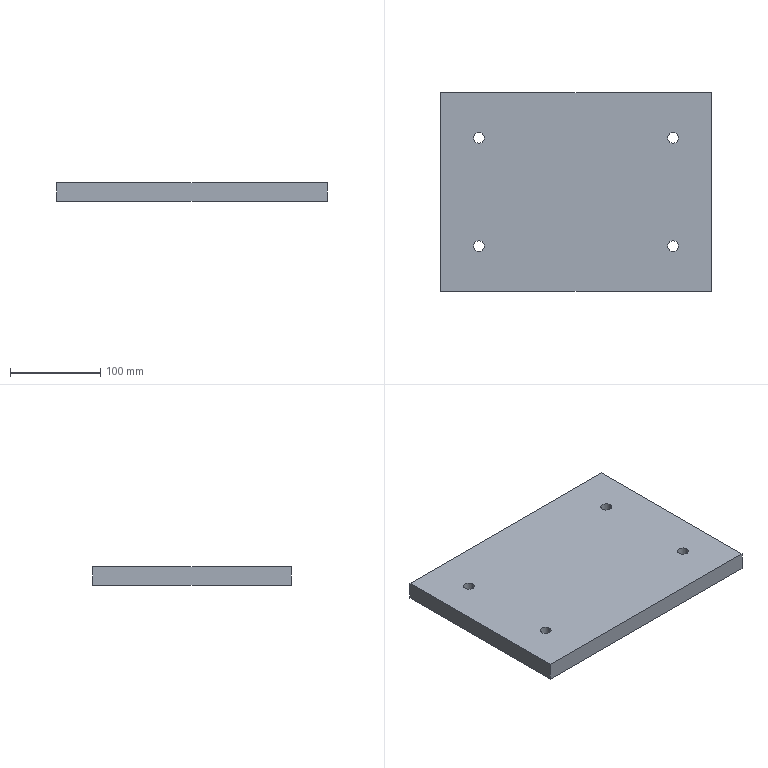Part | STEP file | 000 | 1 solid | 14 faces | box 300 x 220 x 20 mm | volume 1310952 mm3 | cylinder 8 | plane 6 | commonest cylinder face diameters 12 x8
STEP:
#1=CARTESIAN_POINT('',(0.,0.,0.));
#2=DIRECTION('',(0.,0.,1.));
#3=DIRECTION('',(1.,0.,0.));
#4=AXIS2_PLACEMENT_3D('',#1,#2,#3);
#5=CARTESIAN_POINT('',(-150.,110.,0.));
#6=VERTEX_POINT('',#5);
#7=CARTESIAN_POINT('',(-150.,-110.,0.));
#8=VERTEX_POINT('',#7);
#9=CARTESIAN_POINT('',(-150.,110.,0.));
#10=DIRECTION('',(0.,-1.,0.));
#11=VECTOR('',#10,1.);
#12=LINE('',#9,#11);
#13=CARTESIAN_POINT('',(0.,0.,0.));
#14=DIRECTION('',(0.,0.,1.));
#15=DIRECTION('',(1.,0.,0.));
#16=AXIS2_PLACEMENT_3D('',#13,#14,#15);
#17=PLANE('',#16);
#18=CARTESIAN_POINT('',(-150.,110.));
#19=DIRECTION('',(0.,-1.));
#20=VECTOR('',#19,1.);
#21=LINE('',#18,#20);
#22=(GEOMETRIC_REPRESENTATION_CONTEXT(2)PARAMETRIC_REPRESENTATION_CONTEXT()REPRESENTATION_CONTEXT('',''));
#23=DEFINITIONAL_REPRESENTATION('',(#21),#22);
#24=PCURVE('',#17,#23);
#25=CARTESIAN_POINT('',(-150.,0.,10.));
#26=DIRECTION('',(1.,0.,0.));
#27=DIRECTION('',(0.,-1.,0.));
#28=AXIS2_PLACEMENT_3D('',#25,#26,#27);
#29=PLANE('',#28);
#30=CARTESIAN_POINT('',(-110.,10.));
#31=DIRECTION('',(1.,0.));
#32=VECTOR('',#31,1.);
#33=LINE('',#30,#32);
#34=(GEOMETRIC_REPRESENTATION_CONTEXT(2)PARAMETRIC_REPRESENTATION_CONTEXT()REPRESENTATION_CONTEXT('',''));
#35=DEFINITIONAL_REPRESENTATION('',(#33),#34);
#36=PCURVE('',#29,#35);
#37=SURFACE_CURVE('',#12,(#24,#36),.PCURVE_S1.);
#38=EDGE_CURVE('',#6,#8,#37,.T.);
#39=ORIENTED_EDGE('',*,*,#38,.T.);
#40=CARTESIAN_POINT('',(150.,-110.,0.));
#41=VERTEX_POINT('',#40);
#42=CARTESIAN_POINT('',(-150.,-110.,0.));
#43=DIRECTION('',(1.,0.,0.));
#44=VECTOR('',#43,1.);
#45=LINE('',#42,#44);
#46=CARTESIAN_POINT('',(-150.,-110.));
#47=DIRECTION('',(1.,0.));
#48=VECTOR('',#47,1.);
#49=LINE('',#46,#48);
#50=(GEOMETRIC_REPRESENTATION_CONTEXT(2)PARAMETRIC_REPRESENTATION_CONTEXT()REPRESENTATION_CONTEXT('',''));
#51=DEFINITIONAL_REPRESENTATION('',(#49),#50);
#52=PCURVE('',#17,#51);
#53=CARTESIAN_POINT('',(0.,-110.,10.));
#54=DIRECTION('',(0.,1.,0.));
#55=DIRECTION('',(1.,0.,0.));
#56=AXIS2_PLACEMENT_3D('',#53,#54,#55);
#57=PLANE('',#56);
#58=CARTESIAN_POINT('',(-150.,10.));
#59=DIRECTION('',(1.,0.));
#60=VECTOR('',#59,1.);
#61=LINE('',#58,#60);
#62=(GEOMETRIC_REPRESENTATION_CONTEXT(2)PARAMETRIC_REPRESENTATION_CONTEXT()REPRESENTATION_CONTEXT('',''));
#63=DEFINITIONAL_REPRESENTATION('',(#61),#62);
#64=PCURVE('',#57,#63);
#65=SURFACE_CURVE('',#45,(#52,#64),.PCURVE_S1.);
#66=EDGE_CURVE('',#8,#41,#65,.T.);
#67=ORIENTED_EDGE('',*,*,#66,.T.);
#68=CARTESIAN_POINT('',(150.,110.,0.));
#69=VERTEX_POINT('',#68);
#70=CARTESIAN_POINT('',(150.,-110.,0.));
#71=DIRECTION('',(0.,1.,0.));
#72=VECTOR('',#71,1.);
#73=LINE('',#70,#72);
#74=CARTESIAN_POINT('',(150.,-110.));
#75=DIRECTION('',(0.,1.));
#76=VECTOR('',#75,1.);
#77=LINE('',#74,#76);
#78=(GEOMETRIC_REPRESENTATION_CONTEXT(2)PARAMETRIC_REPRESENTATION_CONTEXT()REPRESENTATION_CONTEXT('',''));
#79=DEFINITIONAL_REPRESENTATION('',(#77),#78);
#80=PCURVE('',#17,#79);
#81=CARTESIAN_POINT('',(150.,0.,10.));
#82=DIRECTION('',(-1.,0.,0.));
#83=DIRECTION('',(0.,1.,0.));
#84=AXIS2_PLACEMENT_3D('',#81,#82,#83);
#85=PLANE('',#84);
#86=CARTESIAN_POINT('',(-110.,10.));
#87=DIRECTION('',(1.,0.));
#88=VECTOR('',#87,1.);
#89=LINE('',#86,#88);
#90=(GEOMETRIC_REPRESENTATION_CONTEXT(2)PARAMETRIC_REPRESENTATION_CONTEXT()REPRESENTATION_CONTEXT('',''));
#91=DEFINITIONAL_REPRESENTATION('',(#89),#90);
#92=PCURVE('',#85,#91);
#93=SURFACE_CURVE('',#73,(#80,#92),.PCURVE_S1.);
#94=EDGE_CURVE('',#41,#69,#93,.T.);
#95=ORIENTED_EDGE('',*,*,#94,.T.);
#96=CARTESIAN_POINT('',(150.,110.,0.));
#97=DIRECTION('',(-1.,0.,0.));
#98=VECTOR('',#97,1.);
#99=LINE('',#96,#98);
#100=CARTESIAN_POINT('',(150.,110.));
#101=DIRECTION('',(-1.,0.));
#102=VECTOR('',#101,1.);
#103=LINE('',#100,#102);
#104=(GEOMETRIC_REPRESENTATION_CONTEXT(2)PARAMETRIC_REPRESENTATION_CONTEXT()REPRESENTATION_CONTEXT('',''));
#105=DEFINITIONAL_REPRESENTATION('',(#103),#104);
#106=PCURVE('',#17,#105);
#107=CARTESIAN_POINT('',(0.,110.,10.));
#108=DIRECTION('',(0.,-1.,0.));
#109=DIRECTION('',(-1.,0.,0.));
#110=AXIS2_PLACEMENT_3D('',#107,#108,#109);
#111=PLANE('',#110);
#112=CARTESIAN_POINT('',(-150.,10.));
#113=DIRECTION('',(1.,0.));
#114=VECTOR('',#113,1.);
#115=LINE('',#112,#114);
#116=(GEOMETRIC_REPRESENTATION_CONTEXT(2)PARAMETRIC_REPRESENTATION_CONTEXT()REPRESENTATION_CONTEXT('',''));
#117=DEFINITIONAL_REPRESENTATION('',(#115),#116);
#118=PCURVE('',#111,#117);
#119=SURFACE_CURVE('',#99,(#106,#118),.PCURVE_S1.);
#120=EDGE_CURVE('',#69,#6,#119,.T.);
#121=ORIENTED_EDGE('',*,*,#120,.T.);
#122=EDGE_LOOP('',(#39,#67,#95,#121));
#123=FACE_BOUND('',#122,.F.);
#124=CARTESIAN_POINT('',(-113.5,60.,0.));
#125=VERTEX_POINT('',#124);
#126=CARTESIAN_POINT('',(-101.5,60.,0.));
#127=VERTEX_POINT('',#126);
#128=CARTESIAN_POINT('',(-107.5,60.,0.));
#129=DIRECTION('',(0.,0.,-1.));
#130=DIRECTION('',(-1.,0.,0.));
#131=AXIS2_PLACEMENT_3D('',#128,#129,#130);
#132=CIRCLE('',#131,6.);
#133=CARTESIAN_POINT('',(-113.5,60.));
#134=CARTESIAN_POINT('',(-113.5,70.392));
#135=CARTESIAN_POINT('',(-104.5,65.196));
#136=CARTESIAN_POINT('',(-95.5,60.));
#137=CARTESIAN_POINT('',(-104.5,54.804));
#138=CARTESIAN_POINT('',(-113.5,49.608));
#139=CARTESIAN_POINT('',(-113.5,60.));
#140=(BOUNDED_CURVE()B_SPLINE_CURVE(2,(#133,#134,#135,#136,#137,#138,#139),.UNSPECIFIED.,.T.,.F.)B_SPLINE_CURVE_WITH_KNOTS((1,2,2,2,2,1),(-2.094,0.,2.094,4.189,6.283,8.378),.UNSPECIFIED.)CURVE()GEOMETRIC_REPRESENTATION_ITEM()RATIONAL_B_SPLINE_CURVE((1.,0.5,1.,0.5,1.,0.5,1.))REPRESENTATION_ITEM(''));
#141=(GEOMETRIC_REPRESENTATION_CONTEXT(2)PARAMETRIC_REPRESENTATION_CONTEXT()REPRESENTATION_CONTEXT('',''));
#142=DEFINITIONAL_REPRESENTATION('',(#140),#141);
#143=PCURVE('',#17,#142);
#144=CARTESIAN_POINT('',(-107.5,60.,20.));
#145=DIRECTION('',(0.,0.,-1.));
#146=DIRECTION('',(-1.,0.,0.));
#147=AXIS2_PLACEMENT_3D('',#144,#145,#146);
#148=CYLINDRICAL_SURFACE('',#147,6.);
#149=CARTESIAN_POINT('',(0.,20.));
#150=DIRECTION('',(1.,0.));
#151=VECTOR('',#150,1.);
#152=LINE('',#149,#151);
#153=(GEOMETRIC_REPRESENTATION_CONTEXT(2)PARAMETRIC_REPRESENTATION_CONTEXT()REPRESENTATION_CONTEXT('',''));
#154=DEFINITIONAL_REPRESENTATION('',(#152),#153);
#155=PCURVE('',#148,#154);
#156=SURFACE_CURVE('',#132,(#143,#155),.PCURVE_S1.);
#157=EDGE_CURVE('',#125,#127,#156,.T.);
#158=ORIENTED_EDGE('',*,*,#157,.T.);
#159=CARTESIAN_POINT('',(-107.5,60.,0.));
#160=DIRECTION('',(0.,0.,-1.));
#161=DIRECTION('',(1.,0.,0.));
#162=AXIS2_PLACEMENT_3D('',#159,#160,#161);
#163=CIRCLE('',#162,6.);
#164=CARTESIAN_POINT('',(-101.5,60.));
#165=CARTESIAN_POINT('',(-101.5,49.608));
#166=CARTESIAN_POINT('',(-110.5,54.804));
#167=CARTESIAN_POINT('',(-119.5,60.));
#168=CARTESIAN_POINT('',(-110.5,65.196));
#169=CARTESIAN_POINT('',(-101.5,70.392));
#170=CARTESIAN_POINT('',(-101.5,60.));
#171=(BOUNDED_CURVE()B_SPLINE_CURVE(2,(#164,#165,#166,#167,#168,#169,#170),.UNSPECIFIED.,.T.,.F.)B_SPLINE_CURVE_WITH_KNOTS((1,2,2,2,2,1),(-2.094,0.,2.094,4.189,6.283,8.378),.UNSPECIFIED.)CURVE()GEOMETRIC_REPRESENTATION_ITEM()RATIONAL_B_SPLINE_CURVE((1.,0.5,1.,0.5,1.,0.5,1.))REPRESENTATION_ITEM(''));
#172=(GEOMETRIC_REPRESENTATION_CONTEXT(2)PARAMETRIC_REPRESENTATION_CONTEXT()REPRESENTATION_CONTEXT('',''));
#173=DEFINITIONAL_REPRESENTATION('',(#171),#172);
#174=PCURVE('',#17,#173);
#175=CARTESIAN_POINT('',(-107.5,60.,20.));
#176=DIRECTION('',(0.,0.,-1.));
#177=DIRECTION('',(-1.,0.,0.));
#178=AXIS2_PLACEMENT_3D('',#175,#176,#177);
#179=CYLINDRICAL_SURFACE('',#178,6.);
#180=CARTESIAN_POINT('',(3.142,20.));
#181=DIRECTION('',(1.,0.));
#182=VECTOR('',#181,1.);
#183=LINE('',#180,#182);
#184=(GEOMETRIC_REPRESENTATION_CONTEXT(2)PARAMETRIC_REPRESENTATION_CONTEXT()REPRESENTATION_CONTEXT('',''));
#185=DEFINITIONAL_REPRESENTATION('',(#183),#184);
#186=PCURVE('',#179,#185);
#187=SURFACE_CURVE('',#163,(#174,#186),.PCURVE_S1.);
#188=EDGE_CURVE('',#127,#125,#187,.T.);
#189=ORIENTED_EDGE('',*,*,#188,.T.);
#190=EDGE_LOOP('',(#158,#189));
#191=FACE_BOUND('',#190,.F.);
#192=CARTESIAN_POINT('',(101.5,60.,0.));
#193=VERTEX_POINT('',#192);
#194=CARTESIAN_POINT('',(113.5,60.,0.));
#195=VERTEX_POINT('',#194);
#196=CARTESIAN_POINT('',(107.5,60.,0.));
#197=DIRECTION('',(0.,0.,-1.));
#198=DIRECTION('',(-1.,0.,0.));
#199=AXIS2_PLACEMENT_3D('',#196,#197,#198);
#200=CIRCLE('',#199,6.);
#201=CARTESIAN_POINT('',(101.5,60.));
#202=CARTESIAN_POINT('',(101.5,70.392));
#203=CARTESIAN_POINT('',(110.5,65.196));
#204=CARTESIAN_POINT('',(119.5,60.));
#205=CARTESIAN_POINT('',(110.5,54.804));
#206=CARTESIAN_POINT('',(101.5,49.608));
#207=CARTESIAN_POINT('',(101.5,60.));
#208=(BOUNDED_CURVE()B_SPLINE_CURVE(2,(#201,#202,#203,#204,#205,#206,#207),.UNSPECIFIED.,.T.,.F.)B_SPLINE_CURVE_WITH_KNOTS((1,2,2,2,2,1),(-2.094,0.,2.094,4.189,6.283,8.378),.UNSPECIFIED.)CURVE()GEOMETRIC_REPRESENTATION_ITEM()RATIONAL_B_SPLINE_CURVE((1.,0.5,1.,0.5,1.,0.5,1.))REPRESENTATION_ITEM(''));
#209=(GEOMETRIC_REPRESENTATION_CONTEXT(2)PARAMETRIC_REPRESENTATION_CONTEXT()REPRESENTATION_CONTEXT('',''));
#210=DEFINITIONAL_REPRESENTATION('',(#208),#209);
#211=PCURVE('',#17,#210);
#212=CARTESIAN_POINT('',(107.5,60.,20.));
#213=DIRECTION('',(0.,0.,-1.));
#214=DIRECTION('',(-1.,0.,0.));
#215=AXIS2_PLACEMENT_3D('',#212,#213,#214);
#216=CYLINDRICAL_SURFACE('',#215,6.);
#217=CARTESIAN_POINT('',(0.,20.));
#218=DIRECTION('',(1.,0.));
#219=VECTOR('',#218,1.);
#220=LINE('',#217,#219);
#221=(GEOMETRIC_REPRESENTATION_CONTEXT(2)PARAMETRIC_REPRESENTATION_CONTEXT()REPRESENTATION_CONTEXT('',''));
#222=DEFINITIONAL_REPRESENTATION('',(#220),#221);
#223=PCURVE('',#216,#222);
#224=SURFACE_CURVE('',#200,(#211,#223),.PCURVE_S1.);
#225=EDGE_CURVE('',#193,#195,#224,.T.);
#226=ORIENTED_EDGE('',*,*,#225,.T.);
#227=CARTESIAN_POINT('',(107.5,60.,0.));
#228=DIRECTION('',(0.,0.,-1.));
#229=DIRECTION('',(1.,0.,0.));
#230=AXIS2_PLACEMENT_3D('',#227,#228,#229);
#231=CIRCLE('',#230,6.);
#232=CARTESIAN_POINT('',(113.5,60.));
#233=CARTESIAN_POINT('',(113.5,49.608));
#234=CARTESIAN_POINT('',(104.5,54.804));
#235=CARTESIAN_POINT('',(95.5,60.));
#236=CARTESIAN_POINT('',(104.5,65.196));
#237=CARTESIAN_POINT('',(113.5,70.392));
#238=CARTESIAN_POINT('',(113.5,60.));
#239=(BOUNDED_CURVE()B_SPLINE_CURVE(2,(#232,#233,#234,#235,#236,#237,#238),.UNSPECIFIED.,.T.,.F.)B_SPLINE_CURVE_WITH_KNOTS((1,2,2,2,2,1),(-2.094,0.,2.094,4.189,6.283,8.378),.UNSPECIFIED.)CURVE()GEOMETRIC_REPRESENTATION_ITEM()RATIONAL_B_SPLINE_CURVE((1.,0.5,1.,0.5,1.,0.5,1.))REPRESENTATION_ITEM(''));
#240=(GEOMETRIC_REPRESENTATION_CONTEXT(2)PARAMETRIC_REPRESENTATION_CONTEXT()REPRESENTATION_CONTEXT('',''));
#241=DEFINITIONAL_REPRESENTATION('',(#239),#240);
#242=PCURVE('',#17,#241);
#243=CARTESIAN_POINT('',(107.5,60.,20.));
#244=DIRECTION('',(0.,0.,-1.));
#245=DIRECTION('',(-1.,0.,0.));
#246=AXIS2_PLACEMENT_3D('',#243,#244,#245);
#247=CYLINDRICAL_SURFACE('',#246,6.);
#248=CARTESIAN_POINT('',(3.142,20.));
#249=DIRECTION('',(1.,0.));
#250=VECTOR('',#249,1.);
#251=LINE('',#248,#250);
#252=(GEOMETRIC_REPRESENTATION_CONTEXT(2)PARAMETRIC_REPRESENTATION_CONTEXT()REPRESENTATION_CONTEXT('',''));
#253=DEFINITIONAL_REPRESENTATION('',(#251),#252);
#254=PCURVE('',#247,#253);
#255=SURFACE_CURVE('',#231,(#242,#254),.PCURVE_S1.);
#256=EDGE_CURVE('',#195,#193,#255,.T.);
#257=ORIENTED_EDGE('',*,*,#256,.T.);
#258=EDGE_LOOP('',(#226,#257));
#259=FACE_BOUND('',#258,.F.);
#260=CARTESIAN_POINT('',(-113.5,-60.,0.));
#261=VERTEX_POINT('',#260);
#262=CARTESIAN_POINT('',(-101.5,-60.,0.));
#263=VERTEX_POINT('',#262);
#264=CARTESIAN_POINT('',(-107.5,-60.,0.));
#265=DIRECTION('',(0.,0.,-1.));
#266=DIRECTION('',(-1.,0.,0.));
#267=AXIS2_PLACEMENT_3D('',#264,#265,#266);
#268=CIRCLE('',#267,6.);
#269=CARTESIAN_POINT('',(-113.5,-60.));
#270=CARTESIAN_POINT('',(-113.5,-49.608));
#271=CARTESIAN_POINT('',(-104.5,-54.804));
#272=CARTESIAN_POINT('',(-95.5,-60.));
#273=CARTESIAN_POINT('',(-104.5,-65.196));
#274=CARTESIAN_POINT('',(-113.5,-70.392));
#275=CARTESIAN_POINT('',(-113.5,-60.));
#276=(BOUNDED_CURVE()B_SPLINE_CURVE(2,(#269,#270,#271,#272,#273,#274,#275),.UNSPECIFIED.,.T.,.F.)B_SPLINE_CURVE_WITH_KNOTS((1,2,2,2,2,1),(-2.094,0.,2.094,4.189,6.283,8.378),.UNSPECIFIED.)CURVE()GEOMETRIC_REPRESENTATION_ITEM()RATIONAL_B_SPLINE_CURVE((1.,0.5,1.,0.5,1.,0.5,1.))REPRESENTATION_ITEM(''));
#277=(GEOMETRIC_REPRESENTATION_CONTEXT(2)PARAMETRIC_REPRESENTATION_CONTEXT()REPRESENTATION_CONTEXT('',''));
#278=DEFINITIONAL_REPRESENTATION('',(#276),#277);
#279=PCURVE('',#17,#278);
#280=CARTESIAN_POINT('',(-107.5,-60.,20.));
#281=DIRECTION('',(0.,0.,-1.));
#282=DIRECTION('',(-1.,0.,0.));
#283=AXIS2_PLACEMENT_3D('',#280,#281,#282);
#284=CYLINDRICAL_SURFACE('',#283,6.);
#285=CARTESIAN_POINT('',(0.,20.));
#286=DIRECTION('',(1.,0.));
#287=VECTOR('',#286,1.);
#288=LINE('',#285,#287);
#289=(GEOMETRIC_REPRESENTATION_CONTEXT(2)PARAMETRIC_REPRESENTATION_CONTEXT()REPRESENTATION_CONTEXT('',''));
#290=DEFINITIONAL_REPRESENTATION('',(#288),#289);
#291=PCURVE('',#284,#290);
#292=SURFACE_CURVE('',#268,(#279,#291),.PCURVE_S1.);
#293=EDGE_CURVE('',#261,#263,#292,.T.);
#294=ORIENTED_EDGE('',*,*,#293,.T.);
#295=CARTESIAN_POINT('',(-107.5,-60.,0.));
#296=DIRECTION('',(0.,0.,-1.));
#297=DIRECTION('',(1.,0.,0.));
#298=AXIS2_PLACEMENT_3D('',#295,#296,#297);
#299=CIRCLE('',#298,6.);
#300=CARTESIAN_POINT('',(-101.5,-60.));
#301=CARTESIAN_POINT('',(-101.5,-70.392));
#302=CARTESIAN_POINT('',(-110.5,-65.196));
#303=CARTESIAN_POINT('',(-119.5,-60.));
#304=CARTESIAN_POINT('',(-110.5,-54.804));
#305=CARTESIAN_POINT('',(-101.5,-49.608));
#306=CARTESIAN_POINT('',(-101.5,-60.));
#307=(BOUNDED_CURVE()B_SPLINE_CURVE(2,(#300,#301,#302,#303,#304,#305,#306),.UNSPECIFIED.,.T.,.F.)B_SPLINE_CURVE_WITH_KNOTS((1,2,2,2,2,1),(-2.094,0.,2.094,4.189,6.283,8.378),.UNSPECIFIED.)CURVE()GEOMETRIC_REPRESENTATION_ITEM()RATIONAL_B_SPLINE_CURVE((1.,0.5,1.,0.5,1.,0.5,1.))REPRESENTATION_ITEM(''));
#308=(GEOMETRIC_REPRESENTATION_CONTEXT(2)PARAMETRIC_REPRESENTATION_CONTEXT()REPRESENTATION_CONTEXT('',''));
#309=DEFINITIONAL_REPRESENTATION('',(#307),#308);
#310=PCURVE('',#17,#309);
#311=CARTESIAN_POINT('',(-107.5,-60.,20.));
#312=DIRECTION('',(0.,0.,-1.));
#313=DIRECTION('',(-1.,0.,0.));
#314=AXIS2_PLACEMENT_3D('',#311,#312,#313);
#315=CYLINDRICAL_SURFACE('',#314,6.);
#316=CARTESIAN_POINT('',(3.142,20.));
#317=DIRECTION('',(1.,0.));
#318=VECTOR('',#317,1.);
#319=LINE('',#316,#318);
#320=(GEOMETRIC_REPRESENTATION_CONTEXT(2)PARAMETRIC_REPRESENTATION_CONTEXT()REPRESENTATION_CONTEXT('',''));
#321=DEFINITIONAL_REPRESENTATION('',(#319),#320);
#322=PCURVE('',#315,#321);
#323=SURFACE_CURVE('',#299,(#310,#322),.PCURVE_S1.);
#324=EDGE_CURVE('',#263,#261,#323,.T.);
#325=ORIENTED_EDGE('',*,*,#324,.T.);
#326=EDGE_LOOP('',(#294,#325));
#327=FACE_BOUND('',#326,.F.);
#328=CARTESIAN_POINT('',(101.5,-60.,0.));
#329=VERTEX_POINT('',#328);
#330=CARTESIAN_POINT('',(113.5,-60.,0.));
#331=VERTEX_POINT('',#330);
#332=CARTESIAN_POINT('',(107.5,-60.,0.));
#333=DIRECTION('',(0.,0.,-1.));
#334=DIRECTION('',(-1.,0.,0.));
#335=AXIS2_PLACEMENT_3D('',#332,#333,#334);
#336=CIRCLE('',#335,6.);
#337=CARTESIAN_POINT('',(101.5,-60.));
#338=CARTESIAN_POINT('',(101.5,-49.608));
#339=CARTESIAN_POINT('',(110.5,-54.804));
#340=CARTESIAN_POINT('',(119.5,-60.));
#341=CARTESIAN_POINT('',(110.5,-65.196));
#342=CARTESIAN_POINT('',(101.5,-70.392));
#343=CARTESIAN_POINT('',(101.5,-60.));
#344=(BOUNDED_CURVE()B_SPLINE_CURVE(2,(#337,#338,#339,#340,#341,#342,#343),.UNSPECIFIED.,.T.,.F.)B_SPLINE_CURVE_WITH_KNOTS((1,2,2,2,2,1),(-2.094,0.,2.094,4.189,6.283,8.378),.UNSPECIFIED.)CURVE()GEOMETRIC_REPRESENTATION_ITEM()RATIONAL_B_SPLINE_CURVE((1.,0.5,1.,0.5,1.,0.5,1.))REPRESENTATION_ITEM(''));
#345=(GEOMETRIC_REPRESENTATION_CONTEXT(2)PARAMETRIC_REPRESENTATION_CONTEXT()REPRESENTATION_CONTEXT('',''));
#346=DEFINITIONAL_REPRESENTATION('',(#344),#345);
#347=PCURVE('',#17,#346);
#348=CARTESIAN_POINT('',(107.5,-60.,20.));
#349=DIRECTION('',(0.,0.,-1.));
#350=DIRECTION('',(-1.,0.,0.));
#351=AXIS2_PLACEMENT_3D('',#348,#349,#350);
#352=CYLINDRICAL_SURFACE('',#351,6.);
#353=CARTESIAN_POINT('',(0.,20.));
#354=DIRECTION('',(1.,0.));
#355=VECTOR('',#354,1.);
#356=LINE('',#353,#355);
#357=(GEOMETRIC_REPRESENTATION_CONTEXT(2)PARAMETRIC_REPRESENTATION_CONTEXT()REPRESENTATION_CONTEXT('',''));
#358=DEFINITIONAL_REPRESENTATION('',(#356),#357);
#359=PCURVE('',#352,#358);
#360=SURFACE_CURVE('',#336,(#347,#359),.PCURVE_S1.);
#361=EDGE_CURVE('',#329,#331,#360,.T.);
#362=ORIENTED_EDGE('',*,*,#361,.T.);
#363=CARTESIAN_POINT('',(107.5,-60.,0.));
#364=DIRECTION('',(0.,0.,-1.));
#365=DIRECTION('',(1.,0.,0.));
#366=AXIS2_PLACEMENT_3D('',#363,#364,#365);
#367=CIRCLE('',#366,6.);
#368=CARTESIAN_POINT('',(113.5,-60.));
#369=CARTESIAN_POINT('',(113.5,-70.392));
#370=CARTESIAN_POINT('',(104.5,-65.196));
#371=CARTESIAN_POINT('',(95.5,-60.));
#372=CARTESIAN_POINT('',(104.5,-54.804));
#373=CARTESIAN_POINT('',(113.5,-49.608));
#374=CARTESIAN_POINT('',(113.5,-60.));
#375=(BOUNDED_CURVE()B_SPLINE_CURVE(2,(#368,#369,#370,#371,#372,#373,#374),.UNSPECIFIED.,.T.,.F.)B_SPLINE_CURVE_WITH_KNOTS((1,2,2,2,2,1),(-2.094,0.,2.094,4.189,6.283,8.378),.UNSPECIFIED.)CURVE()GEOMETRIC_REPRESENTATION_ITEM()RATIONAL_B_SPLINE_CURVE((1.,0.5,1.,0.5,1.,0.5,1.))REPRESENTATION_ITEM(''));
#376=(GEOMETRIC_REPRESENTATION_CONTEXT(2)PARAMETRIC_REPRESENTATION_CONTEXT()REPRESENTATION_CONTEXT('',''));
#377=DEFINITIONAL_REPRESENTATION('',(#375),#376);
#378=PCURVE('',#17,#377);
#379=CARTESIAN_POINT('',(107.5,-60.,20.));
#380=DIRECTION('',(0.,0.,-1.));
#381=DIRECTION('',(-1.,0.,0.));
#382=AXIS2_PLACEMENT_3D('',#379,#380,#381);
#383=CYLINDRICAL_SURFACE('',#382,6.);
#384=CARTESIAN_POINT('',(3.142,20.));
#385=DIRECTION('',(1.,0.));
#386=VECTOR('',#385,1.);
#387=LINE('',#384,#386);
#388=(GEOMETRIC_REPRESENTATION_CONTEXT(2)PARAMETRIC_REPRESENTATION_CONTEXT()REPRESENTATION_CONTEXT('',''));
#389=DEFINITIONAL_REPRESENTATION('',(#387),#388);
#390=PCURVE('',#383,#389);
#391=SURFACE_CURVE('',#367,(#378,#390),.PCURVE_S1.);
#392=EDGE_CURVE('',#331,#329,#391,.T.);
#393=ORIENTED_EDGE('',*,*,#392,.T.);
#394=EDGE_LOOP('',(#362,#393));
#395=FACE_BOUND('',#394,.F.);
#396=ADVANCED_FACE('',(#123,#191,#259,#327,#395),#17,.F.);
#397=ORIENTED_EDGE('',*,*,#38,.F.);
#398=CARTESIAN_POINT('',(-150.,110.,20.));
#399=VERTEX_POINT('',#398);
#400=CARTESIAN_POINT('',(-150.,110.,0.));
#401=DIRECTION('',(0.,0.,1.));
#402=VECTOR('',#401,1.);
#403=LINE('',#400,#402);
#404=CARTESIAN_POINT('',(-110.,10.));
#405=DIRECTION('',(0.,-1.));
#406=VECTOR('',#405,1.);
#407=LINE('',#404,#406);
#408=(GEOMETRIC_REPRESENTATION_CONTEXT(2)PARAMETRIC_REPRESENTATION_CONTEXT()REPRESENTATION_CONTEXT('',''));
#409=DEFINITIONAL_REPRESENTATION('',(#407),#408);
#410=PCURVE('',#29,#409);
#411=CARTESIAN_POINT('',(150.,10.));
#412=DIRECTION('',(0.,-1.));
#413=VECTOR('',#412,1.);
#414=LINE('',#411,#413);
#415=(GEOMETRIC_REPRESENTATION_CONTEXT(2)PARAMETRIC_REPRESENTATION_CONTEXT()REPRESENTATION_CONTEXT('',''));
#416=DEFINITIONAL_REPRESENTATION('',(#414),#415);
#417=PCURVE('',#111,#416);
#418=SURFACE_CURVE('',#403,(#410,#417),.PCURVE_S1.);
#419=EDGE_CURVE('',#6,#399,#418,.T.);
#420=ORIENTED_EDGE('',*,*,#419,.T.);
#421=CARTESIAN_POINT('',(-150.,-110.,20.));
#422=VERTEX_POINT('',#421);
#423=CARTESIAN_POINT('',(-150.,110.,20.));
#424=DIRECTION('',(0.,-1.,0.));
#425=VECTOR('',#424,1.);
#426=LINE('',#423,#425);
#427=CARTESIAN_POINT('',(-110.,-10.));
#428=DIRECTION('',(1.,0.));
#429=VECTOR('',#428,1.);
#430=LINE('',#427,#429);
#431=(GEOMETRIC_REPRESENTATION_CONTEXT(2)PARAMETRIC_REPRESENTATION_CONTEXT()REPRESENTATION_CONTEXT('',''));
#432=DEFINITIONAL_REPRESENTATION('',(#430),#431);
#433=PCURVE('',#29,#432);
#434=CARTESIAN_POINT('',(0.,0.,20.));
#435=DIRECTION('',(0.,0.,1.));
#436=DIRECTION('',(1.,0.,0.));
#437=AXIS2_PLACEMENT_3D('',#434,#435,#436);
#438=PLANE('',#437);
#439=CARTESIAN_POINT('',(-150.,110.));
#440=DIRECTION('',(0.,-1.));
#441=VECTOR('',#440,1.);
#442=LINE('',#439,#441);
#443=(GEOMETRIC_REPRESENTATION_CONTEXT(2)PARAMETRIC_REPRESENTATION_CONTEXT()REPRESENTATION_CONTEXT('',''));
#444=DEFINITIONAL_REPRESENTATION('',(#442),#443);
#445=PCURVE('',#438,#444);
#446=SURFACE_CURVE('',#426,(#433,#445),.PCURVE_S1.);
#447=EDGE_CURVE('',#399,#422,#446,.T.);
#448=ORIENTED_EDGE('',*,*,#447,.T.);
#449=CARTESIAN_POINT('',(-150.,-110.,0.));
#450=DIRECTION('',(0.,0.,1.));
#451=VECTOR('',#450,1.);
#452=LINE('',#449,#451);
#453=CARTESIAN_POINT('',(110.,10.));
#454=DIRECTION('',(0.,-1.));
#455=VECTOR('',#454,1.);
#456=LINE('',#453,#455);
#457=(GEOMETRIC_REPRESENTATION_CONTEXT(2)PARAMETRIC_REPRESENTATION_CONTEXT()REPRESENTATION_CONTEXT('',''));
#458=DEFINITIONAL_REPRESENTATION('',(#456),#457);
#459=PCURVE('',#29,#458);
#460=CARTESIAN_POINT('',(-150.,10.));
#461=DIRECTION('',(0.,-1.));
#462=VECTOR('',#461,1.);
#463=LINE('',#460,#462);
#464=(GEOMETRIC_REPRESENTATION_CONTEXT(2)PARAMETRIC_REPRESENTATION_CONTEXT()REPRESENTATION_CONTEXT('',''));
#465=DEFINITIONAL_REPRESENTATION('',(#463),#464);
#466=PCURVE('',#57,#465);
#467=SURFACE_CURVE('',#452,(#459,#466),.PCURVE_S1.);
#468=EDGE_CURVE('',#8,#422,#467,.T.);
#469=ORIENTED_EDGE('',*,*,#468,.F.);
#470=EDGE_LOOP('',(#397,#420,#448,#469));
#471=FACE_BOUND('',#470,.F.);
#472=ADVANCED_FACE('',(#471),#29,.F.);
#473=ORIENTED_EDGE('',*,*,#120,.F.);
#474=CARTESIAN_POINT('',(150.,110.,20.));
#475=VERTEX_POINT('',#474);
#476=CARTESIAN_POINT('',(150.,110.,0.));
#477=DIRECTION('',(0.,0.,1.));
#478=VECTOR('',#477,1.);
#479=LINE('',#476,#478);
#480=CARTESIAN_POINT('',(-150.,10.));
#481=DIRECTION('',(0.,-1.));
#482=VECTOR('',#481,1.);
#483=LINE('',#480,#482);
#484=(GEOMETRIC_REPRESENTATION_CONTEXT(2)PARAMETRIC_REPRESENTATION_CONTEXT()REPRESENTATION_CONTEXT('',''));
#485=DEFINITIONAL_REPRESENTATION('',(#483),#484);
#486=PCURVE('',#111,#485);
#487=CARTESIAN_POINT('',(110.,10.));
#488=DIRECTION('',(0.,-1.));
#489=VECTOR('',#488,1.);
#490=LINE('',#487,#489);
#491=(GEOMETRIC_REPRESENTATION_CONTEXT(2)PARAMETRIC_REPRESENTATION_CONTEXT()REPRESENTATION_CONTEXT('',''));
#492=DEFINITIONAL_REPRESENTATION('',(#490),#491);
#493=PCURVE('',#85,#492);
#494=SURFACE_CURVE('',#479,(#486,#493),.PCURVE_S1.);
#495=EDGE_CURVE('',#69,#475,#494,.T.);
#496=ORIENTED_EDGE('',*,*,#495,.T.);
#497=CARTESIAN_POINT('',(150.,110.,20.));
#498=DIRECTION('',(-1.,0.,0.));
#499=VECTOR('',#498,1.);
#500=LINE('',#497,#499);
#501=CARTESIAN_POINT('',(-150.,-10.));
#502=DIRECTION('',(1.,0.));
#503=VECTOR('',#502,1.);
#504=LINE('',#501,#503);
#505=(GEOMETRIC_REPRESENTATION_CONTEXT(2)PARAMETRIC_REPRESENTATION_CONTEXT()REPRESENTATION_CONTEXT('',''));
#506=DEFINITIONAL_REPRESENTATION('',(#504),#505);
#507=PCURVE('',#111,#506);
#508=CARTESIAN_POINT('',(150.,110.));
#509=DIRECTION('',(-1.,0.));
#510=VECTOR('',#509,1.);
#511=LINE('',#508,#510);
#512=(GEOMETRIC_REPRESENTATION_CONTEXT(2)PARAMETRIC_REPRESENTATION_CONTEXT()REPRESENTATION_CONTEXT('',''));
#513=DEFINITIONAL_REPRESENTATION('',(#511),#512);
#514=PCURVE('',#438,#513);
#515=SURFACE_CURVE('',#500,(#507,#514),.PCURVE_S1.);
#516=EDGE_CURVE('',#475,#399,#515,.T.);
#517=ORIENTED_EDGE('',*,*,#516,.T.);
#518=ORIENTED_EDGE('',*,*,#419,.F.);
#519=EDGE_LOOP('',(#473,#496,#517,#518));
#520=FACE_BOUND('',#519,.F.);
#521=ADVANCED_FACE('',(#520),#111,.F.);
#522=ORIENTED_EDGE('',*,*,#94,.F.);
#523=CARTESIAN_POINT('',(150.,-110.,20.));
#524=VERTEX_POINT('',#523);
#525=CARTESIAN_POINT('',(150.,-110.,0.));
#526=DIRECTION('',(0.,0.,1.));
#527=VECTOR('',#526,1.);
#528=LINE('',#525,#527);
#529=CARTESIAN_POINT('',(-110.,10.));
#530=DIRECTION('',(0.,-1.));
#531=VECTOR('',#530,1.);
#532=LINE('',#529,#531);
#533=(GEOMETRIC_REPRESENTATION_CONTEXT(2)PARAMETRIC_REPRESENTATION_CONTEXT()REPRESENTATION_CONTEXT('',''));
#534=DEFINITIONAL_REPRESENTATION('',(#532),#533);
#535=PCURVE('',#85,#534);
#536=CARTESIAN_POINT('',(150.,10.));
#537=DIRECTION('',(0.,-1.));
#538=VECTOR('',#537,1.);
#539=LINE('',#536,#538);
#540=(GEOMETRIC_REPRESENTATION_CONTEXT(2)PARAMETRIC_REPRESENTATION_CONTEXT()REPRESENTATION_CONTEXT('',''));
#541=DEFINITIONAL_REPRESENTATION('',(#539),#540);
#542=PCURVE('',#57,#541);
#543=SURFACE_CURVE('',#528,(#535,#542),.PCURVE_S1.);
#544=EDGE_CURVE('',#41,#524,#543,.T.);
#545=ORIENTED_EDGE('',*,*,#544,.T.);
#546=CARTESIAN_POINT('',(150.,-110.,20.));
#547=DIRECTION('',(0.,1.,0.));
#548=VECTOR('',#547,1.);
#549=LINE('',#546,#548);
#550=CARTESIAN_POINT('',(-110.,-10.));
#551=DIRECTION('',(1.,0.));
#552=VECTOR('',#551,1.);
#553=LINE('',#550,#552);
#554=(GEOMETRIC_REPRESENTATION_CONTEXT(2)PARAMETRIC_REPRESENTATION_CONTEXT()REPRESENTATION_CONTEXT('',''));
#555=DEFINITIONAL_REPRESENTATION('',(#553),#554);
#556=PCURVE('',#85,#555);
#557=CARTESIAN_POINT('',(150.,-110.));
#558=DIRECTION('',(0.,1.));
#559=VECTOR('',#558,1.);
#560=LINE('',#557,#559);
#561=(GEOMETRIC_REPRESENTATION_CONTEXT(2)PARAMETRIC_REPRESENTATION_CONTEXT()REPRESENTATION_CONTEXT('',''));
#562=DEFINITIONAL_REPRESENTATION('',(#560),#561);
#563=PCURVE('',#438,#562);
#564=SURFACE_CURVE('',#549,(#556,#563),.PCURVE_S1.);
#565=EDGE_CURVE('',#524,#475,#564,.T.);
#566=ORIENTED_EDGE('',*,*,#565,.T.);
#567=ORIENTED_EDGE('',*,*,#495,.F.);
#568=EDGE_LOOP('',(#522,#545,#566,#567));
#569=FACE_BOUND('',#568,.F.);
#570=ADVANCED_FACE('',(#569),#85,.F.);
#571=ORIENTED_EDGE('',*,*,#66,.F.);
#572=ORIENTED_EDGE('',*,*,#468,.T.);
#573=CARTESIAN_POINT('',(-150.,-110.,20.));
#574=DIRECTION('',(1.,0.,0.));
#575=VECTOR('',#574,1.);
#576=LINE('',#573,#575);
#577=CARTESIAN_POINT('',(-150.,-10.));
#578=DIRECTION('',(1.,0.));
#579=VECTOR('',#578,1.);
#580=LINE('',#577,#579);
#581=(GEOMETRIC_REPRESENTATION_CONTEXT(2)PARAMETRIC_REPRESENTATION_CONTEXT()REPRESENTATION_CONTEXT('',''));
#582=DEFINITIONAL_REPRESENTATION('',(#580),#581);
#583=PCURVE('',#57,#582);
#584=CARTESIAN_POINT('',(-150.,-110.));
#585=DIRECTION('',(1.,0.));
#586=VECTOR('',#585,1.);
#587=LINE('',#584,#586);
#588=(GEOMETRIC_REPRESENTATION_CONTEXT(2)PARAMETRIC_REPRESENTATION_CONTEXT()REPRESENTATION_CONTEXT('',''));
#589=DEFINITIONAL_REPRESENTATION('',(#587),#588);
#590=PCURVE('',#438,#589);
#591=SURFACE_CURVE('',#576,(#583,#590),.PCURVE_S1.);
#592=EDGE_CURVE('',#422,#524,#591,.T.);
#593=ORIENTED_EDGE('',*,*,#592,.T.);
#594=ORIENTED_EDGE('',*,*,#544,.F.);
#595=EDGE_LOOP('',(#571,#572,#593,#594));
#596=FACE_BOUND('',#595,.F.);
#597=ADVANCED_FACE('',(#596),#57,.F.);
#598=ORIENTED_EDGE('',*,*,#447,.F.);
#599=ORIENTED_EDGE('',*,*,#516,.F.);
#600=ORIENTED_EDGE('',*,*,#565,.F.);
#601=ORIENTED_EDGE('',*,*,#592,.F.);
#602=EDGE_LOOP('',(#598,#599,#600,#601));
#603=FACE_BOUND('',#602,.F.);
#604=CARTESIAN_POINT('',(-113.5,60.,20.));
#605=VERTEX_POINT('',#604);
#606=CARTESIAN_POINT('',(-101.5,60.,20.));
#607=VERTEX_POINT('',#606);
#608=CARTESIAN_POINT('',(-107.5,60.,20.));
#609=DIRECTION('',(0.,0.,-1.));
#610=DIRECTION('',(-1.,0.,0.));
#611=AXIS2_PLACEMENT_3D('',#608,#609,#610);
#612=CIRCLE('',#611,6.);
#613=CARTESIAN_POINT('',(-113.5,60.));
#614=CARTESIAN_POINT('',(-113.5,70.392));
#615=CARTESIAN_POINT('',(-104.5,65.196));
#616=CARTESIAN_POINT('',(-95.5,60.));
#617=CARTESIAN_POINT('',(-104.5,54.804));
#618=CARTESIAN_POINT('',(-113.5,49.608));
#619=CARTESIAN_POINT('',(-113.5,60.));
#620=(BOUNDED_CURVE()B_SPLINE_CURVE(2,(#613,#614,#615,#616,#617,#618,#619),.UNSPECIFIED.,.T.,.F.)B_SPLINE_CURVE_WITH_KNOTS((1,2,2,2,2,1),(-2.094,0.,2.094,4.189,6.283,8.378),.UNSPECIFIED.)CURVE()GEOMETRIC_REPRESENTATION_ITEM()RATIONAL_B_SPLINE_CURVE((1.,0.5,1.,0.5,1.,0.5,1.))REPRESENTATION_ITEM(''));
#621=(GEOMETRIC_REPRESENTATION_CONTEXT(2)PARAMETRIC_REPRESENTATION_CONTEXT()REPRESENTATION_CONTEXT('',''));
#622=DEFINITIONAL_REPRESENTATION('',(#620),#621);
#623=PCURVE('',#438,#622);
#624=CARTESIAN_POINT('',(0.,0.));
#625=DIRECTION('',(1.,0.));
#626=VECTOR('',#625,1.);
#627=LINE('',#624,#626);
#628=(GEOMETRIC_REPRESENTATION_CONTEXT(2)PARAMETRIC_REPRESENTATION_CONTEXT()REPRESENTATION_CONTEXT('',''));
#629=DEFINITIONAL_REPRESENTATION('',(#627),#628);
#630=PCURVE('',#148,#629);
#631=SURFACE_CURVE('',#612,(#623,#630),.PCURVE_S1.);
#632=EDGE_CURVE('',#605,#607,#631,.T.);
#633=ORIENTED_EDGE('',*,*,#632,.F.);
#634=CARTESIAN_POINT('',(-107.5,60.,20.));
#635=DIRECTION('',(0.,0.,-1.));
#636=DIRECTION('',(1.,0.,0.));
#637=AXIS2_PLACEMENT_3D('',#634,#635,#636);
#638=CIRCLE('',#637,6.);
#639=CARTESIAN_POINT('',(-101.5,60.));
#640=CARTESIAN_POINT('',(-101.5,49.608));
#641=CARTESIAN_POINT('',(-110.5,54.804));
#642=CARTESIAN_POINT('',(-119.5,60.));
#643=CARTESIAN_POINT('',(-110.5,65.196));
#644=CARTESIAN_POINT('',(-101.5,70.392));
#645=CARTESIAN_POINT('',(-101.5,60.));
#646=(BOUNDED_CURVE()B_SPLINE_CURVE(2,(#639,#640,#641,#642,#643,#644,#645),.UNSPECIFIED.,.T.,.F.)B_SPLINE_CURVE_WITH_KNOTS((1,2,2,2,2,1),(-2.094,0.,2.094,4.189,6.283,8.378),.UNSPECIFIED.)CURVE()GEOMETRIC_REPRESENTATION_ITEM()RATIONAL_B_SPLINE_CURVE((1.,0.5,1.,0.5,1.,0.5,1.))REPRESENTATION_ITEM(''));
#647=(GEOMETRIC_REPRESENTATION_CONTEXT(2)PARAMETRIC_REPRESENTATION_CONTEXT()REPRESENTATION_CONTEXT('',''));
#648=DEFINITIONAL_REPRESENTATION('',(#646),#647);
#649=PCURVE('',#438,#648);
#650=CARTESIAN_POINT('',(3.142,0.));
#651=DIRECTION('',(1.,0.));
#652=VECTOR('',#651,1.);
#653=LINE('',#650,#652);
#654=(GEOMETRIC_REPRESENTATION_CONTEXT(2)PARAMETRIC_REPRESENTATION_CONTEXT()REPRESENTATION_CONTEXT('',''));
#655=DEFINITIONAL_REPRESENTATION('',(#653),#654);
#656=PCURVE('',#179,#655);
#657=SURFACE_CURVE('',#638,(#649,#656),.PCURVE_S1.);
#658=EDGE_CURVE('',#607,#605,#657,.T.);
#659=ORIENTED_EDGE('',*,*,#658,.F.);
#660=EDGE_LOOP('',(#633,#659));
#661=FACE_BOUND('',#660,.F.);
#662=CARTESIAN_POINT('',(101.5,60.,20.));
#663=VERTEX_POINT('',#662);
#664=CARTESIAN_POINT('',(113.5,60.,20.));
#665=VERTEX_POINT('',#664);
#666=CARTESIAN_POINT('',(107.5,60.,20.));
#667=DIRECTION('',(0.,0.,-1.));
#668=DIRECTION('',(-1.,0.,0.));
#669=AXIS2_PLACEMENT_3D('',#666,#667,#668);
#670=CIRCLE('',#669,6.);
#671=CARTESIAN_POINT('',(101.5,60.));
#672=CARTESIAN_POINT('',(101.5,70.392));
#673=CARTESIAN_POINT('',(110.5,65.196));
#674=CARTESIAN_POINT('',(119.5,60.));
#675=CARTESIAN_POINT('',(110.5,54.804));
#676=CARTESIAN_POINT('',(101.5,49.608));
#677=CARTESIAN_POINT('',(101.5,60.));
#678=(BOUNDED_CURVE()B_SPLINE_CURVE(2,(#671,#672,#673,#674,#675,#676,#677),.UNSPECIFIED.,.T.,.F.)B_SPLINE_CURVE_WITH_KNOTS((1,2,2,2,2,1),(-2.094,0.,2.094,4.189,6.283,8.378),.UNSPECIFIED.)CURVE()GEOMETRIC_REPRESENTATION_ITEM()RATIONAL_B_SPLINE_CURVE((1.,0.5,1.,0.5,1.,0.5,1.))REPRESENTATION_ITEM(''));
#679=(GEOMETRIC_REPRESENTATION_CONTEXT(2)PARAMETRIC_REPRESENTATION_CONTEXT()REPRESENTATION_CONTEXT('',''));
#680=DEFINITIONAL_REPRESENTATION('',(#678),#679);
#681=PCURVE('',#438,#680);
#682=CARTESIAN_POINT('',(0.,0.));
#683=DIRECTION('',(1.,0.));
#684=VECTOR('',#683,1.);
#685=LINE('',#682,#684);
#686=(GEOMETRIC_REPRESENTATION_CONTEXT(2)PARAMETRIC_REPRESENTATION_CONTEXT()REPRESENTATION_CONTEXT('',''));
#687=DEFINITIONAL_REPRESENTATION('',(#685),#686);
#688=PCURVE('',#216,#687);
#689=SURFACE_CURVE('',#670,(#681,#688),.PCURVE_S1.);
#690=EDGE_CURVE('',#663,#665,#689,.T.);
#691=ORIENTED_EDGE('',*,*,#690,.F.);
#692=CARTESIAN_POINT('',(107.5,60.,20.));
#693=DIRECTION('',(0.,0.,-1.));
#694=DIRECTION('',(1.,0.,0.));
#695=AXIS2_PLACEMENT_3D('',#692,#693,#694);
#696=CIRCLE('',#695,6.);
#697=CARTESIAN_POINT('',(113.5,60.));
#698=CARTESIAN_POINT('',(113.5,49.608));
#699=CARTESIAN_POINT('',(104.5,54.804));
#700=CARTESIAN_POINT('',(95.5,60.));
#701=CARTESIAN_POINT('',(104.5,65.196));
#702=CARTESIAN_POINT('',(113.5,70.392));
#703=CARTESIAN_POINT('',(113.5,60.));
#704=(BOUNDED_CURVE()B_SPLINE_CURVE(2,(#697,#698,#699,#700,#701,#702,#703),.UNSPECIFIED.,.T.,.F.)B_SPLINE_CURVE_WITH_KNOTS((1,2,2,2,2,1),(-2.094,0.,2.094,4.189,6.283,8.378),.UNSPECIFIED.)CURVE()GEOMETRIC_REPRESENTATION_ITEM()RATIONAL_B_SPLINE_CURVE((1.,0.5,1.,0.5,1.,0.5,1.))REPRESENTATION_ITEM(''));
#705=(GEOMETRIC_REPRESENTATION_CONTEXT(2)PARAMETRIC_REPRESENTATION_CONTEXT()REPRESENTATION_CONTEXT('',''));
#706=DEFINITIONAL_REPRESENTATION('',(#704),#705);
#707=PCURVE('',#438,#706);
#708=CARTESIAN_POINT('',(3.142,0.));
#709=DIRECTION('',(1.,0.));
#710=VECTOR('',#709,1.);
#711=LINE('',#708,#710);
#712=(GEOMETRIC_REPRESENTATION_CONTEXT(2)PARAMETRIC_REPRESENTATION_CONTEXT()REPRESENTATION_CONTEXT('',''));
#713=DEFINITIONAL_REPRESENTATION('',(#711),#712);
#714=PCURVE('',#247,#713);
#715=SURFACE_CURVE('',#696,(#707,#714),.PCURVE_S1.);
#716=EDGE_CURVE('',#665,#663,#715,.T.);
#717=ORIENTED_EDGE('',*,*,#716,.F.);
#718=EDGE_LOOP('',(#691,#717));
#719=FACE_BOUND('',#718,.F.);
#720=CARTESIAN_POINT('',(-113.5,-60.,20.));
#721=VERTEX_POINT('',#720);
#722=CARTESIAN_POINT('',(-101.5,-60.,20.));
#723=VERTEX_POINT('',#722);
#724=CARTESIAN_POINT('',(-107.5,-60.,20.));
#725=DIRECTION('',(0.,0.,-1.));
#726=DIRECTION('',(-1.,0.,0.));
#727=AXIS2_PLACEMENT_3D('',#724,#725,#726);
#728=CIRCLE('',#727,6.);
#729=CARTESIAN_POINT('',(-113.5,-60.));
#730=CARTESIAN_POINT('',(-113.5,-49.608));
#731=CARTESIAN_POINT('',(-104.5,-54.804));
#732=CARTESIAN_POINT('',(-95.5,-60.));
#733=CARTESIAN_POINT('',(-104.5,-65.196));
#734=CARTESIAN_POINT('',(-113.5,-70.392));
#735=CARTESIAN_POINT('',(-113.5,-60.));
#736=(BOUNDED_CURVE()B_SPLINE_CURVE(2,(#729,#730,#731,#732,#733,#734,#735),.UNSPECIFIED.,.T.,.F.)B_SPLINE_CURVE_WITH_KNOTS((1,2,2,2,2,1),(-2.094,0.,2.094,4.189,6.283,8.378),.UNSPECIFIED.)CURVE()GEOMETRIC_REPRESENTATION_ITEM()RATIONAL_B_SPLINE_CURVE((1.,0.5,1.,0.5,1.,0.5,1.))REPRESENTATION_ITEM(''));
#737=(GEOMETRIC_REPRESENTATION_CONTEXT(2)PARAMETRIC_REPRESENTATION_CONTEXT()REPRESENTATION_CONTEXT('',''));
#738=DEFINITIONAL_REPRESENTATION('',(#736),#737);
#739=PCURVE('',#438,#738);
#740=CARTESIAN_POINT('',(0.,0.));
#741=DIRECTION('',(1.,0.));
#742=VECTOR('',#741,1.);
#743=LINE('',#740,#742);
#744=(GEOMETRIC_REPRESENTATION_CONTEXT(2)PARAMETRIC_REPRESENTATION_CONTEXT()REPRESENTATION_CONTEXT('',''));
#745=DEFINITIONAL_REPRESENTATION('',(#743),#744);
#746=PCURVE('',#284,#745);
#747=SURFACE_CURVE('',#728,(#739,#746),.PCURVE_S1.);
#748=EDGE_CURVE('',#721,#723,#747,.T.);
#749=ORIENTED_EDGE('',*,*,#748,.F.);
#750=CARTESIAN_POINT('',(-107.5,-60.,20.));
#751=DIRECTION('',(0.,0.,-1.));
#752=DIRECTION('',(1.,0.,0.));
#753=AXIS2_PLACEMENT_3D('',#750,#751,#752);
#754=CIRCLE('',#753,6.);
#755=CARTESIAN_POINT('',(-101.5,-60.));
#756=CARTESIAN_POINT('',(-101.5,-70.392));
#757=CARTESIAN_POINT('',(-110.5,-65.196));
#758=CARTESIAN_POINT('',(-119.5,-60.));
#759=CARTESIAN_POINT('',(-110.5,-54.804));
#760=CARTESIAN_POINT('',(-101.5,-49.608));
#761=CARTESIAN_POINT('',(-101.5,-60.));
#762=(BOUNDED_CURVE()B_SPLINE_CURVE(2,(#755,#756,#757,#758,#759,#760,#761),.UNSPECIFIED.,.T.,.F.)B_SPLINE_CURVE_WITH_KNOTS((1,2,2,2,2,1),(-2.094,0.,2.094,4.189,6.283,8.378),.UNSPECIFIED.)CURVE()GEOMETRIC_REPRESENTATION_ITEM()RATIONAL_B_SPLINE_CURVE((1.,0.5,1.,0.5,1.,0.5,1.))REPRESENTATION_ITEM(''));
#763=(GEOMETRIC_REPRESENTATION_CONTEXT(2)PARAMETRIC_REPRESENTATION_CONTEXT()REPRESENTATION_CONTEXT('',''));
#764=DEFINITIONAL_REPRESENTATION('',(#762),#763);
#765=PCURVE('',#438,#764);
#766=CARTESIAN_POINT('',(3.142,0.));
#767=DIRECTION('',(1.,0.));
#768=VECTOR('',#767,1.);
#769=LINE('',#766,#768);
#770=(GEOMETRIC_REPRESENTATION_CONTEXT(2)PARAMETRIC_REPRESENTATION_CONTEXT()REPRESENTATION_CONTEXT('',''));
#771=DEFINITIONAL_REPRESENTATION('',(#769),#770);
#772=PCURVE('',#315,#771);
#773=SURFACE_CURVE('',#754,(#765,#772),.PCURVE_S1.);
#774=EDGE_CURVE('',#723,#721,#773,.T.);
#775=ORIENTED_EDGE('',*,*,#774,.F.);
#776=EDGE_LOOP('',(#749,#775));
#777=FACE_BOUND('',#776,.F.);
#778=CARTESIAN_POINT('',(101.5,-60.,20.));
#779=VERTEX_POINT('',#778);
#780=CARTESIAN_POINT('',(113.5,-60.,20.));
#781=VERTEX_POINT('',#780);
#782=CARTESIAN_POINT('',(107.5,-60.,20.));
#783=DIRECTION('',(0.,0.,-1.));
#784=DIRECTION('',(-1.,0.,0.));
#785=AXIS2_PLACEMENT_3D('',#782,#783,#784);
#786=CIRCLE('',#785,6.);
#787=CARTESIAN_POINT('',(101.5,-60.));
#788=CARTESIAN_POINT('',(101.5,-49.608));
#789=CARTESIAN_POINT('',(110.5,-54.804));
#790=CARTESIAN_POINT('',(119.5,-60.));
#791=CARTESIAN_POINT('',(110.5,-65.196));
#792=CARTESIAN_POINT('',(101.5,-70.392));
#793=CARTESIAN_POINT('',(101.5,-60.));
#794=(BOUNDED_CURVE()B_SPLINE_CURVE(2,(#787,#788,#789,#790,#791,#792,#793),.UNSPECIFIED.,.T.,.F.)B_SPLINE_CURVE_WITH_KNOTS((1,2,2,2,2,1),(-2.094,0.,2.094,4.189,6.283,8.378),.UNSPECIFIED.)CURVE()GEOMETRIC_REPRESENTATION_ITEM()RATIONAL_B_SPLINE_CURVE((1.,0.5,1.,0.5,1.,0.5,1.))REPRESENTATION_ITEM(''));
#795=(GEOMETRIC_REPRESENTATION_CONTEXT(2)PARAMETRIC_REPRESENTATION_CONTEXT()REPRESENTATION_CONTEXT('',''));
#796=DEFINITIONAL_REPRESENTATION('',(#794),#795);
#797=PCURVE('',#438,#796);
#798=CARTESIAN_POINT('',(0.,0.));
#799=DIRECTION('',(1.,0.));
#800=VECTOR('',#799,1.);
#801=LINE('',#798,#800);
#802=(GEOMETRIC_REPRESENTATION_CONTEXT(2)PARAMETRIC_REPRESENTATION_CONTEXT()REPRESENTATION_CONTEXT('',''));
#803=DEFINITIONAL_REPRESENTATION('',(#801),#802);
#804=PCURVE('',#352,#803);
#805=SURFACE_CURVE('',#786,(#797,#804),.PCURVE_S1.);
#806=EDGE_CURVE('',#779,#781,#805,.T.);
#807=ORIENTED_EDGE('',*,*,#806,.F.);
#808=CARTESIAN_POINT('',(107.5,-60.,20.));
#809=DIRECTION('',(0.,0.,-1.));
#810=DIRECTION('',(1.,0.,0.));
#811=AXIS2_PLACEMENT_3D('',#808,#809,#810);
#812=CIRCLE('',#811,6.);
#813=CARTESIAN_POINT('',(113.5,-60.));
#814=CARTESIAN_POINT('',(113.5,-70.392));
#815=CARTESIAN_POINT('',(104.5,-65.196));
#816=CARTESIAN_POINT('',(95.5,-60.));
#817=CARTESIAN_POINT('',(104.5,-54.804));
#818=CARTESIAN_POINT('',(113.5,-49.608));
#819=CARTESIAN_POINT('',(113.5,-60.));
#820=(BOUNDED_CURVE()B_SPLINE_CURVE(2,(#813,#814,#815,#816,#817,#818,#819),.UNSPECIFIED.,.T.,.F.)B_SPLINE_CURVE_WITH_KNOTS((1,2,2,2,2,1),(-2.094,0.,2.094,4.189,6.283,8.378),.UNSPECIFIED.)CURVE()GEOMETRIC_REPRESENTATION_ITEM()RATIONAL_B_SPLINE_CURVE((1.,0.5,1.,0.5,1.,0.5,1.))REPRESENTATION_ITEM(''));
#821=(GEOMETRIC_REPRESENTATION_CONTEXT(2)PARAMETRIC_REPRESENTATION_CONTEXT()REPRESENTATION_CONTEXT('',''));
#822=DEFINITIONAL_REPRESENTATION('',(#820),#821);
#823=PCURVE('',#438,#822);
#824=CARTESIAN_POINT('',(3.142,0.));
#825=DIRECTION('',(1.,0.));
#826=VECTOR('',#825,1.);
#827=LINE('',#824,#826);
#828=(GEOMETRIC_REPRESENTATION_CONTEXT(2)PARAMETRIC_REPRESENTATION_CONTEXT()REPRESENTATION_CONTEXT('',''));
#829=DEFINITIONAL_REPRESENTATION('',(#827),#828);
#830=PCURVE('',#383,#829);
#831=SURFACE_CURVE('',#812,(#823,#830),.PCURVE_S1.);
#832=EDGE_CURVE('',#781,#779,#831,.T.);
#833=ORIENTED_EDGE('',*,*,#832,.F.);
#834=EDGE_LOOP('',(#807,#833));
#835=FACE_BOUND('',#834,.F.);
#836=ADVANCED_FACE('',(#603,#661,#719,#777,#835),#438,.T.);
#837=ORIENTED_EDGE('',*,*,#157,.F.);
#838=CARTESIAN_POINT('',(-113.5,60.,20.));
#839=DIRECTION('',(0.,0.,-1.));
#840=VECTOR('',#839,1.);
#841=LINE('',#838,#840);
#842=CARTESIAN_POINT('',(0.,0.));
#843=DIRECTION('',(0.,1.));
#844=VECTOR('',#843,1.);
#845=LINE('',#842,#844);
#846=(GEOMETRIC_REPRESENTATION_CONTEXT(2)PARAMETRIC_REPRESENTATION_CONTEXT()REPRESENTATION_CONTEXT('',''));
#847=DEFINITIONAL_REPRESENTATION('',(#845),#846);
#848=PCURVE('',#148,#847);
#849=CARTESIAN_POINT('',(6.283,0.));
#850=DIRECTION('',(0.,1.));
#851=VECTOR('',#850,1.);
#852=LINE('',#849,#851);
#853=(GEOMETRIC_REPRESENTATION_CONTEXT(2)PARAMETRIC_REPRESENTATION_CONTEXT()REPRESENTATION_CONTEXT('',''));
#854=DEFINITIONAL_REPRESENTATION('',(#852),#853);
#855=PCURVE('',#179,#854);
#856=SURFACE_CURVE('',#841,(#848,#855),.PCURVE_S1.);
#857=EDGE_CURVE('',#605,#125,#856,.T.);
#858=ORIENTED_EDGE('',*,*,#857,.F.);
#859=ORIENTED_EDGE('',*,*,#632,.T.);
#860=CARTESIAN_POINT('',(-101.5,60.,20.));
#861=DIRECTION('',(0.,0.,-1.));
#862=VECTOR('',#861,1.);
#863=LINE('',#860,#862);
#864=CARTESIAN_POINT('',(3.142,0.));
#865=DIRECTION('',(0.,1.));
#866=VECTOR('',#865,1.);
#867=LINE('',#864,#866);
#868=(GEOMETRIC_REPRESENTATION_CONTEXT(2)PARAMETRIC_REPRESENTATION_CONTEXT()REPRESENTATION_CONTEXT('',''));
#869=DEFINITIONAL_REPRESENTATION('',(#867),#868);
#870=PCURVE('',#148,#869);
#871=CARTESIAN_POINT('',(3.142,0.));
#872=DIRECTION('',(0.,1.));
#873=VECTOR('',#872,1.);
#874=LINE('',#871,#873);
#875=(GEOMETRIC_REPRESENTATION_CONTEXT(2)PARAMETRIC_REPRESENTATION_CONTEXT()REPRESENTATION_CONTEXT('',''));
#876=DEFINITIONAL_REPRESENTATION('',(#874),#875);
#877=PCURVE('',#179,#876);
#878=SURFACE_CURVE('',#863,(#870,#877),.PCURVE_S1.);
#879=EDGE_CURVE('',#607,#127,#878,.T.);
#880=ORIENTED_EDGE('',*,*,#879,.T.);
#881=EDGE_LOOP('',(#837,#858,#859,#880));
#882=FACE_BOUND('',#881,.F.);
#883=ADVANCED_FACE('',(#882),#148,.F.);
#884=ORIENTED_EDGE('',*,*,#188,.F.);
#885=ORIENTED_EDGE('',*,*,#879,.F.);
#886=ORIENTED_EDGE('',*,*,#658,.T.);
#887=ORIENTED_EDGE('',*,*,#857,.T.);
#888=EDGE_LOOP('',(#884,#885,#886,#887));
#889=FACE_BOUND('',#888,.F.);
#890=ADVANCED_FACE('',(#889),#179,.F.);
#891=ORIENTED_EDGE('',*,*,#225,.F.);
#892=CARTESIAN_POINT('',(101.5,60.,20.));
#893=DIRECTION('',(0.,0.,-1.));
#894=VECTOR('',#893,1.);
#895=LINE('',#892,#894);
#896=CARTESIAN_POINT('',(0.,0.));
#897=DIRECTION('',(0.,1.));
#898=VECTOR('',#897,1.);
#899=LINE('',#896,#898);
#900=(GEOMETRIC_REPRESENTATION_CONTEXT(2)PARAMETRIC_REPRESENTATION_CONTEXT()REPRESENTATION_CONTEXT('',''));
#901=DEFINITIONAL_REPRESENTATION('',(#899),#900);
#902=PCURVE('',#216,#901);
#903=CARTESIAN_POINT('',(6.283,0.));
#904=DIRECTION('',(0.,1.));
#905=VECTOR('',#904,1.);
#906=LINE('',#903,#905);
#907=(GEOMETRIC_REPRESENTATION_CONTEXT(2)PARAMETRIC_REPRESENTATION_CONTEXT()REPRESENTATION_CONTEXT('',''));
#908=DEFINITIONAL_REPRESENTATION('',(#906),#907);
#909=PCURVE('',#247,#908);
#910=SURFACE_CURVE('',#895,(#902,#909),.PCURVE_S1.);
#911=EDGE_CURVE('',#663,#193,#910,.T.);
#912=ORIENTED_EDGE('',*,*,#911,.F.);
#913=ORIENTED_EDGE('',*,*,#690,.T.);
#914=CARTESIAN_POINT('',(113.5,60.,20.));
#915=DIRECTION('',(0.,0.,-1.));
#916=VECTOR('',#915,1.);
#917=LINE('',#914,#916);
#918=CARTESIAN_POINT('',(3.142,0.));
#919=DIRECTION('',(0.,1.));
#920=VECTOR('',#919,1.);
#921=LINE('',#918,#920);
#922=(GEOMETRIC_REPRESENTATION_CONTEXT(2)PARAMETRIC_REPRESENTATION_CONTEXT()REPRESENTATION_CONTEXT('',''));
#923=DEFINITIONAL_REPRESENTATION('',(#921),#922);
#924=PCURVE('',#216,#923);
#925=CARTESIAN_POINT('',(3.142,0.));
#926=DIRECTION('',(0.,1.));
#927=VECTOR('',#926,1.);
#928=LINE('',#925,#927);
#929=(GEOMETRIC_REPRESENTATION_CONTEXT(2)PARAMETRIC_REPRESENTATION_CONTEXT()REPRESENTATION_CONTEXT('',''));
#930=DEFINITIONAL_REPRESENTATION('',(#928),#929);
#931=PCURVE('',#247,#930);
#932=SURFACE_CURVE('',#917,(#924,#931),.PCURVE_S1.);
#933=EDGE_CURVE('',#665,#195,#932,.T.);
#934=ORIENTED_EDGE('',*,*,#933,.T.);
#935=EDGE_LOOP('',(#891,#912,#913,#934));
#936=FACE_BOUND('',#935,.F.);
#937=ADVANCED_FACE('',(#936),#216,.F.);
#938=ORIENTED_EDGE('',*,*,#256,.F.);
#939=ORIENTED_EDGE('',*,*,#933,.F.);
#940=ORIENTED_EDGE('',*,*,#716,.T.);
#941=ORIENTED_EDGE('',*,*,#911,.T.);
#942=EDGE_LOOP('',(#938,#939,#940,#941));
#943=FACE_BOUND('',#942,.F.);
#944=ADVANCED_FACE('',(#943),#247,.F.);
#945=ORIENTED_EDGE('',*,*,#293,.F.);
#946=CARTESIAN_POINT('',(-113.5,-60.,20.));
#947=DIRECTION('',(0.,0.,-1.));
#948=VECTOR('',#947,1.);
#949=LINE('',#946,#948);
#950=CARTESIAN_POINT('',(0.,0.));
#951=DIRECTION('',(0.,1.));
#952=VECTOR('',#951,1.);
#953=LINE('',#950,#952);
#954=(GEOMETRIC_REPRESENTATION_CONTEXT(2)PARAMETRIC_REPRESENTATION_CONTEXT()REPRESENTATION_CONTEXT('',''));
#955=DEFINITIONAL_REPRESENTATION('',(#953),#954);
#956=PCURVE('',#284,#955);
#957=CARTESIAN_POINT('',(6.283,0.));
#958=DIRECTION('',(0.,1.));
#959=VECTOR('',#958,1.);
#960=LINE('',#957,#959);
#961=(GEOMETRIC_REPRESENTATION_CONTEXT(2)PARAMETRIC_REPRESENTATION_CONTEXT()REPRESENTATION_CONTEXT('',''));
#962=DEFINITIONAL_REPRESENTATION('',(#960),#961);
#963=PCURVE('',#315,#962);
#964=SURFACE_CURVE('',#949,(#956,#963),.PCURVE_S1.);
#965=EDGE_CURVE('',#721,#261,#964,.T.);
#966=ORIENTED_EDGE('',*,*,#965,.F.);
#967=ORIENTED_EDGE('',*,*,#748,.T.);
#968=CARTESIAN_POINT('',(-101.5,-60.,20.));
#969=DIRECTION('',(0.,0.,-1.));
#970=VECTOR('',#969,1.);
#971=LINE('',#968,#970);
#972=CARTESIAN_POINT('',(3.142,0.));
#973=DIRECTION('',(0.,1.));
#974=VECTOR('',#973,1.);
#975=LINE('',#972,#974);
#976=(GEOMETRIC_REPRESENTATION_CONTEXT(2)PARAMETRIC_REPRESENTATION_CONTEXT()REPRESENTATION_CONTEXT('',''));
#977=DEFINITIONAL_REPRESENTATION('',(#975),#976);
#978=PCURVE('',#284,#977);
#979=CARTESIAN_POINT('',(3.142,0.));
#980=DIRECTION('',(0.,1.));
#981=VECTOR('',#980,1.);
#982=LINE('',#979,#981);
#983=(GEOMETRIC_REPRESENTATION_CONTEXT(2)PARAMETRIC_REPRESENTATION_CONTEXT()REPRESENTATION_CONTEXT('',''));
#984=DEFINITIONAL_REPRESENTATION('',(#982),#983);
#985=PCURVE('',#315,#984);
#986=SURFACE_CURVE('',#971,(#978,#985),.PCURVE_S1.);
#987=EDGE_CURVE('',#723,#263,#986,.T.);
#988=ORIENTED_EDGE('',*,*,#987,.T.);
#989=EDGE_LOOP('',(#945,#966,#967,#988));
#990=FACE_BOUND('',#989,.F.);
#991=ADVANCED_FACE('',(#990),#284,.F.);
#992=ORIENTED_EDGE('',*,*,#324,.F.);
#993=ORIENTED_EDGE('',*,*,#987,.F.);
#994=ORIENTED_EDGE('',*,*,#774,.T.);
#995=ORIENTED_EDGE('',*,*,#965,.T.);
#996=EDGE_LOOP('',(#992,#993,#994,#995));
#997=FACE_BOUND('',#996,.F.);
#998=ADVANCED_FACE('',(#997),#315,.F.);
#999=ORIENTED_EDGE('',*,*,#361,.F.);
#1000=CARTESIAN_POINT('',(101.5,-60.,20.));
#1001=DIRECTION('',(0.,0.,-1.));
#1002=VECTOR('',#1001,1.);
#1003=LINE('',#1000,#1002);
#1004=CARTESIAN_POINT('',(0.,0.));
#1005=DIRECTION('',(0.,1.));
#1006=VECTOR('',#1005,1.);
#1007=LINE('',#1004,#1006);
#1008=(GEOMETRIC_REPRESENTATION_CONTEXT(2)PARAMETRIC_REPRESENTATION_CONTEXT()REPRESENTATION_CONTEXT('',''));
#1009=DEFINITIONAL_REPRESENTATION('',(#1007),#1008);
#1010=PCURVE('',#352,#1009);
#1011=CARTESIAN_POINT('',(6.283,0.));
#1012=DIRECTION('',(0.,1.));
#1013=VECTOR('',#1012,1.);
#1014=LINE('',#1011,#1013);
#1015=(GEOMETRIC_REPRESENTATION_CONTEXT(2)PARAMETRIC_REPRESENTATION_CONTEXT()REPRESENTATION_CONTEXT('',''));
#1016=DEFINITIONAL_REPRESENTATION('',(#1014),#1015);
#1017=PCURVE('',#383,#1016);
#1018=SURFACE_CURVE('',#1003,(#1010,#1017),.PCURVE_S1.);
#1019=EDGE_CURVE('',#779,#329,#1018,.T.);
#1020=ORIENTED_EDGE('',*,*,#1019,.F.);
#1021=ORIENTED_EDGE('',*,*,#806,.T.);
#1022=CARTESIAN_POINT('',(113.5,-60.,20.));
#1023=DIRECTION('',(0.,0.,-1.));
#1024=VECTOR('',#1023,1.);
#1025=LINE('',#1022,#1024);
#1026=CARTESIAN_POINT('',(3.142,0.));
#1027=DIRECTION('',(0.,1.));
#1028=VECTOR('',#1027,1.);
#1029=LINE('',#1026,#1028);
#1030=(GEOMETRIC_REPRESENTATION_CONTEXT(2)PARAMETRIC_REPRESENTATION_CONTEXT()REPRESENTATION_CONTEXT('',''));
#1031=DEFINITIONAL_REPRESENTATION('',(#1029),#1030);
#1032=PCURVE('',#352,#1031);
#1033=CARTESIAN_POINT('',(3.142,0.));
#1034=DIRECTION('',(0.,1.));
#1035=VECTOR('',#1034,1.);
#1036=LINE('',#1033,#1035);
#1037=(GEOMETRIC_REPRESENTATION_CONTEXT(2)PARAMETRIC_REPRESENTATION_CONTEXT()REPRESENTATION_CONTEXT('',''));
#1038=DEFINITIONAL_REPRESENTATION('',(#1036),#1037);
#1039=PCURVE('',#383,#1038);
#1040=SURFACE_CURVE('',#1025,(#1032,#1039),.PCURVE_S1.);
#1041=EDGE_CURVE('',#781,#331,#1040,.T.);
#1042=ORIENTED_EDGE('',*,*,#1041,.T.);
#1043=EDGE_LOOP('',(#999,#1020,#1021,#1042));
#1044=FACE_BOUND('',#1043,.F.);
#1045=ADVANCED_FACE('',(#1044),#352,.F.);
#1046=ORIENTED_EDGE('',*,*,#392,.F.);
#1047=ORIENTED_EDGE('',*,*,#1041,.F.);
#1048=ORIENTED_EDGE('',*,*,#832,.T.);
#1049=ORIENTED_EDGE('',*,*,#1019,.T.);
#1050=EDGE_LOOP('',(#1046,#1047,#1048,#1049));
#1051=FACE_BOUND('',#1050,.F.);
#1052=ADVANCED_FACE('',(#1051),#383,.F.);
#1053=CLOSED_SHELL('',(#396,#472,#521,#570,#597,#836,#883,#890,#937,#944,#991,#998,#1045,#1052));
#1054=MANIFOLD_SOLID_BREP('',#1053);
#1055=(LENGTH_UNIT()NAMED_UNIT(*)SI_UNIT(.MILLI.,.METRE.));
#1056=UNCERTAINTY_MEASURE_WITH_UNIT(LENGTH_MEASURE(0.0000001),#1055,'','');
#1057=(NAMED_UNIT(*)PLANE_ANGLE_UNIT()SI_UNIT($,.RADIAN.));
#1058=(NAMED_UNIT(*)SI_UNIT($,.STERADIAN.)SOLID_ANGLE_UNIT());
#1059=(GEOMETRIC_REPRESENTATION_CONTEXT(3)GLOBAL_UNCERTAINTY_ASSIGNED_CONTEXT((#1056))GLOBAL_UNIT_ASSIGNED_CONTEXT((#1055,#1057,#1058))REPRESENTATION_CONTEXT('',''));
#1060=ADVANCED_BREP_SHAPE_REPRESENTATION('',(#4,#1054),#1059);